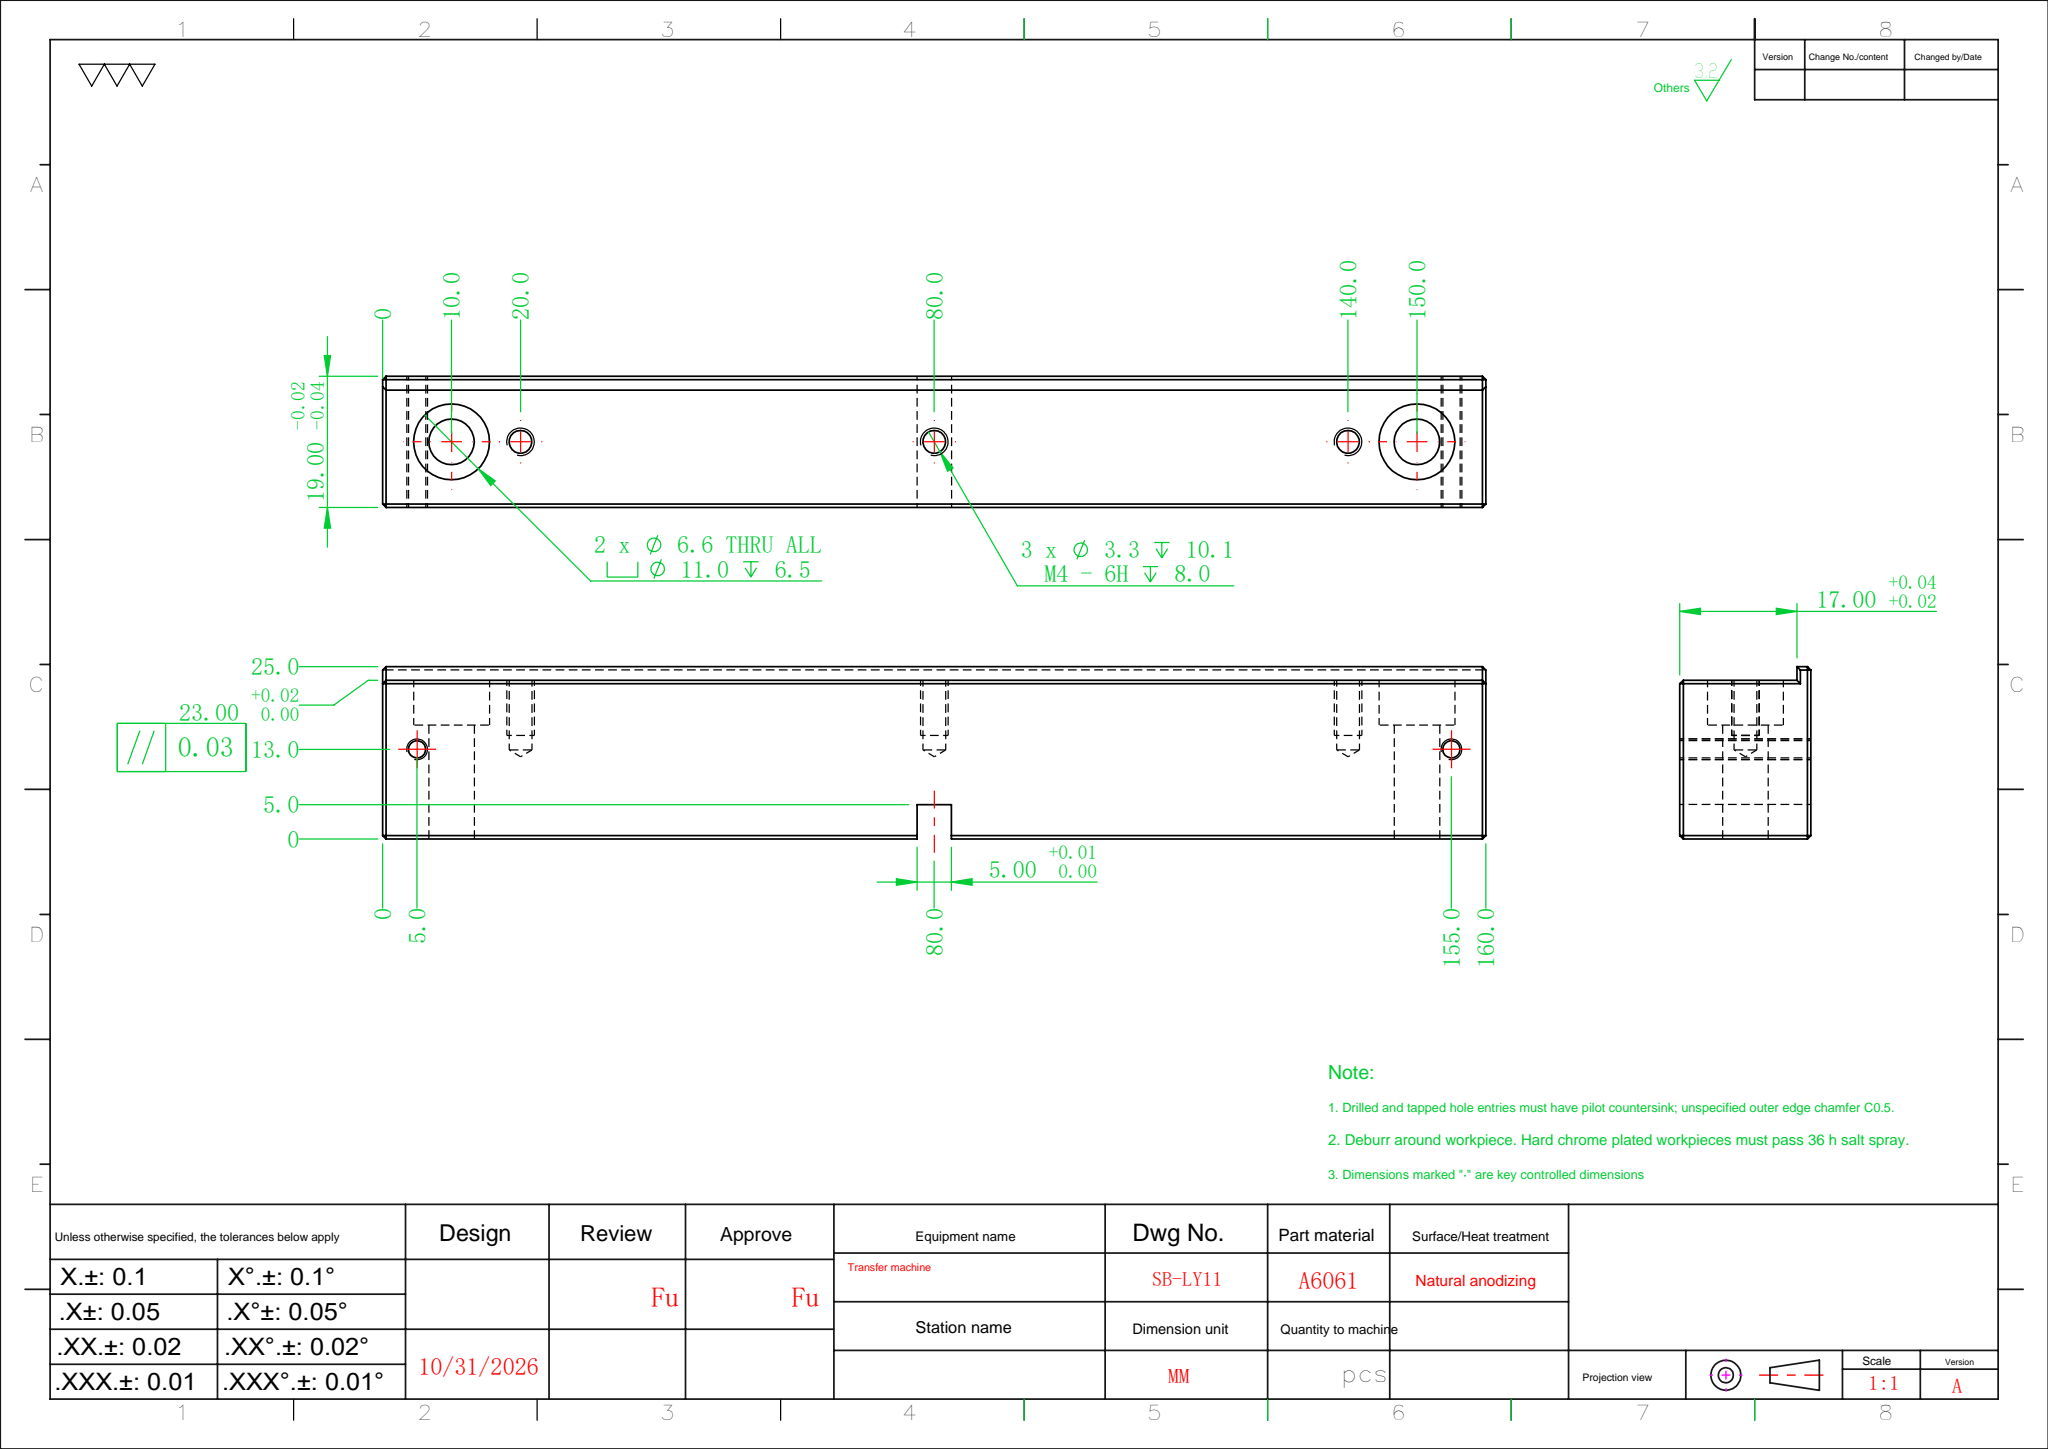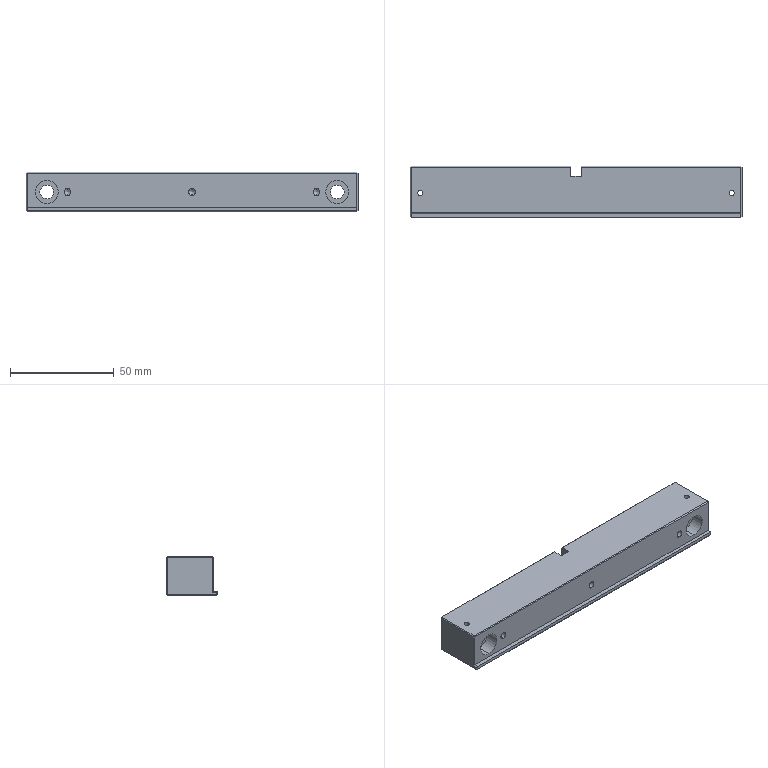Part | SolidWorks | features HoleWzd 3, ICE 2, Chamfer 1, Cut 1, Extrusion 1 | 1 solid | 64 faces | box 160 x 25 x 19 mm | volume 67166 mm3 | plane 40 | cylinder 18 | cone 6 | commonest cylinder face diameters 3.3 x6 2.5 x4 6.6 x4 11 x4